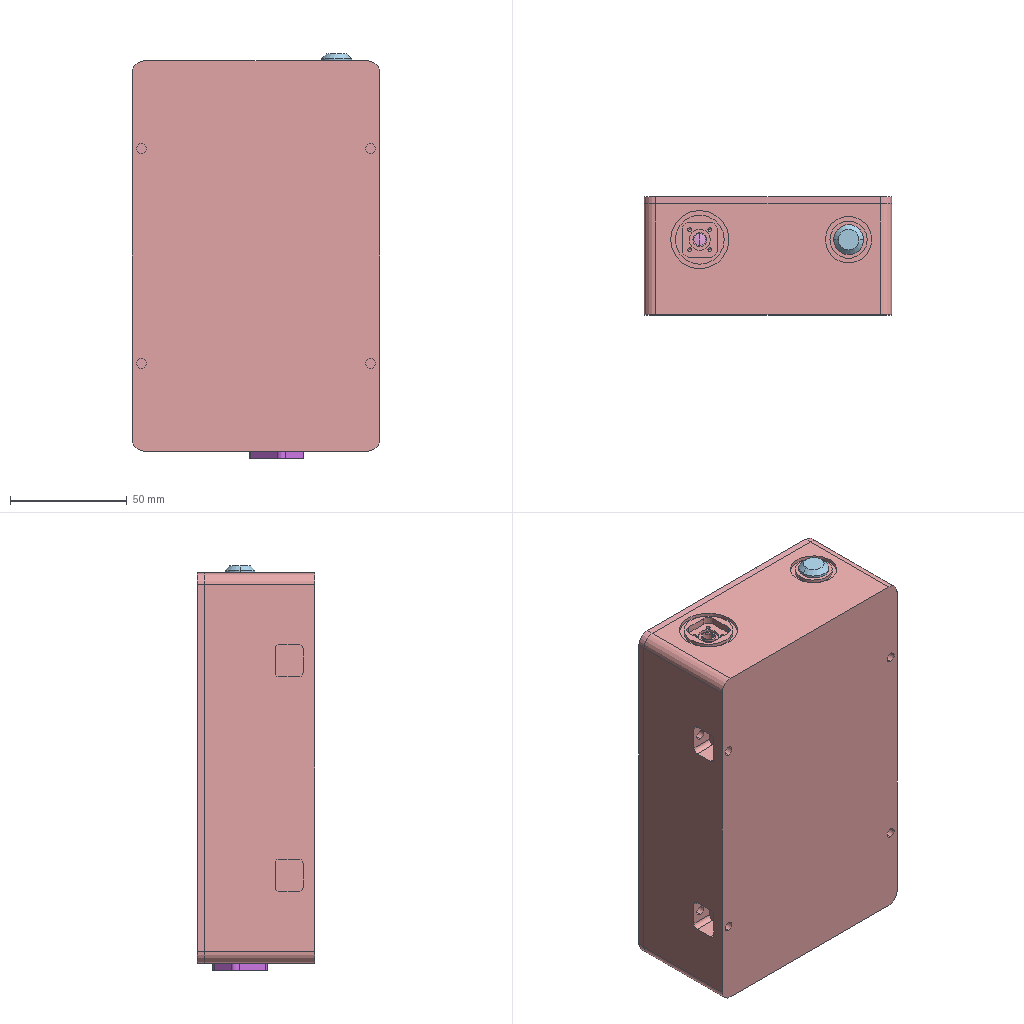Assembly | SolidWorks | 29 different items | 40 placed | box 106 x 50 x 173 mm
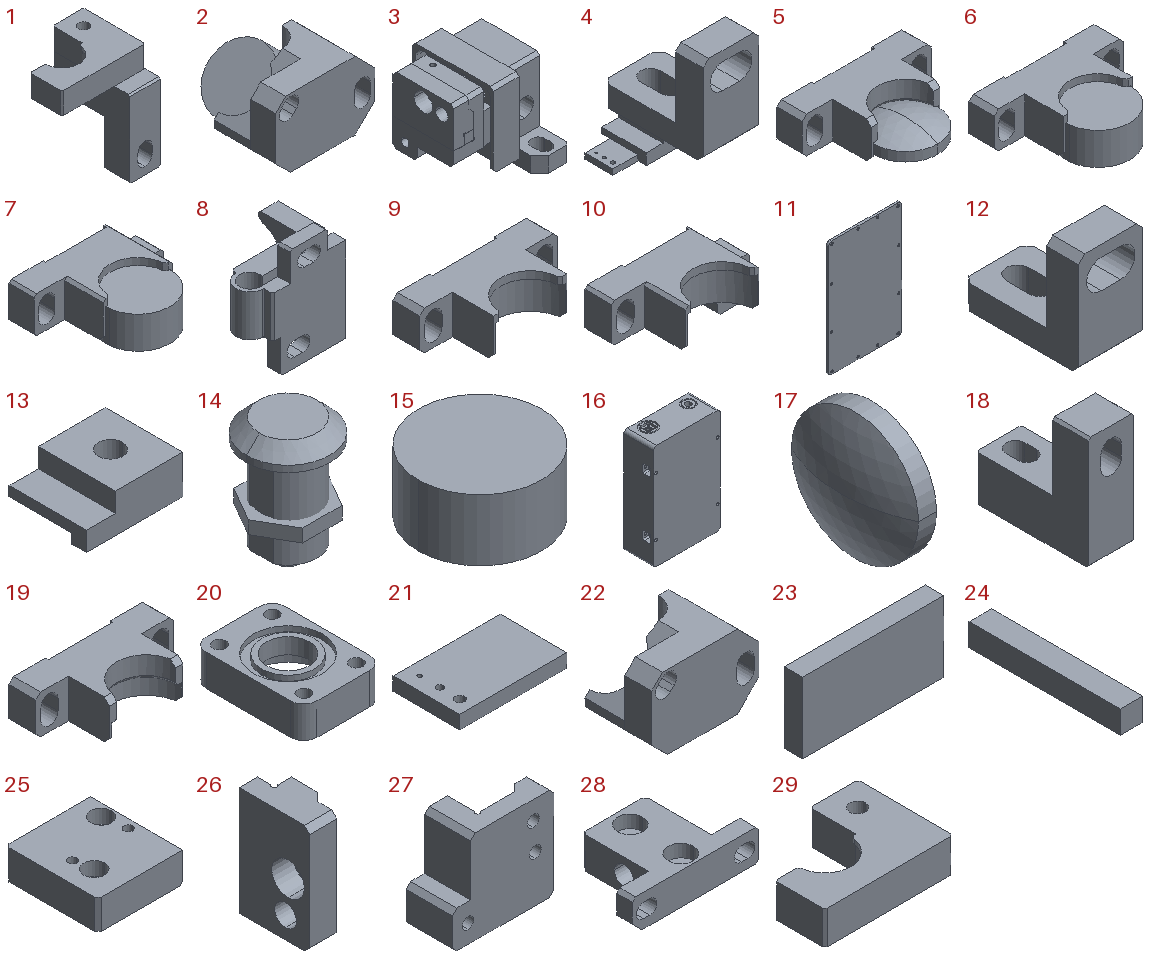Parts list (item | name | quantity | parent item | size | volume | features):
1 | (subassembly) | x1 | - | 26.9 x 25 x 32 mm | 5358 mm3 | -
2 | (subassembly) | x2 | - | 19.9 x 19.05 x 14.189 mm | 2294 mm3 | -
3 | (subassembly) | x1 | - | 27.5 x 40 x 26.65 mm | 12052 mm3 | -
4 | (subassembly) | x1 | - | 16 x 18 x 19.75 mm | 1298 mm3 | -
5 | (subassembly) | x2 | - | 25.6 x 19.05 x 7.31 mm | 1491 mm3 | features CompositeCurve 1
6 | (subassembly) | x2 | - | 25.6 x 19.05 x 7.7 mm | 1838 mm3 | -
7 | (subassembly) | x1 | - | 25.6 x 19.05 x 12.05 mm | 1859 mm3 | -
8 | - | x1 | - | 20.78 x 16.7 x 25 mm | 2347 mm3 | features MoveFace 8, Chamfer 5, ICE 5, BaseBody 1, DelFace 1, Fillet 1
9 | - | x2 | in 6 | 25.6 x 12.7 x 7.2 mm | 1033 mm3 | features ICE 7, Chamfer 3, MoveFace 2, Extrusion 1
10 | - | x1 | in 7 | 25.6 x 12.7 x 12.05 mm | 1054 mm3 | features ICE 7, Chamfer 4, MoveFace 2, Extrusion 1, Fillet 1
11 | - | x1 | - | 106 x 3 x 167 mm | 52528 mm3 | features Extrusion 1, HoleWzd 1
12 | - | x1 | in 4 | 10 x 18 x 15.75 mm | 1032 mm3 | features ICE 4, Chamfer 1, Extrusion 1
13 | - | x1 | in 4 | 10 x 8 x 4 mm | 226.365 mm3 | features ICE 4, Extrusion 1, HoleWzd 1, MoveFace 1
14 | - | x1 | - | 12.9 x 12.9 x 19.1 mm | 1271 mm3 | features ICE 4, Chamfer 1, Extrusion 1
15 | - | x5 | in 2, 6, 7 | 12.7 x 12.7 x 6.35 mm | 804.398 mm3 | features Extrusion 1
16 | - | x1 | - | 106 x 47.3 x 167 mm | 437913 mm3 | features ICE 29, MoveFace 24, HoleWzd 23, Fillet 19, Cut 18, DelFace 18, 3DProfileFeature 1, Extrusion 1, LPattern 1
17 | - | x2 | in 5 | 4.7 x 12.7 x 12.7 mm | 415.033 mm3 | features Revolution 1
18 | - | x1 | in 1 | 10 x 25 x 25 mm | 3226 mm3 | features ICE 3, Chamfer 1, Extrusion 1, MoveFace 1
19 | - | x2 | in 5 | 25.6 x 12.7 x 7.2 mm | 1076 mm3 | features ICE 7, Chamfer 2, MoveFace 2, Extrusion 1, Fillet 1
20 | - | x1 | - | 15 x 21 x 6 mm | 975.148 mm3 | features ICE 5, Extrusion 1, Fillet 1
21 | - | x1 | in 4 | 8 x 5 x 1 mm | 39.348 mm3 | features ICE 2, Extrusion 1
22 | - | x2 | in 2 | 19.9 x 12.7 x 13.659 mm | 1490 mm3 | features ICE 10, Chamfer 3, Extrusion 1, MoveFace 1
23 | - | x1 | in 3 | 20 x 2.6 x 10 mm | 520 mm3 | features Extrusion 1
24 | - | x1 | in 3 | 3 x 20 x 3 mm | 180 mm3 | features Extrusion 1
25 | - | x1 | in 3 | 24.4 x 26.5 x 8.5 mm | 3196 mm3 | features MoveFace 4, Chamfer 2, DelFace 2, HoleWzd 2, Extrusion 1, Fillet 1, ICE 1
26 | - | x1 | in 3 | 6.5 x 13 x 20 mm | 1157 mm3 | features Cut 2, Chamfer 1, Extrusion 1, HoleWzd 1
27 | - | x1 | in 3 | 21.9 x 9.9 x 20 mm | 2171 mm3 | features HoleWzd 3, ICE 2, MoveFace 2, Chamfer 1, Extrusion 1
28 | - | x1 | in 3 | 40 x 26 x 10 mm | 4828 mm3 | features ICE 3, Chamfer 2, Extrusion 1, HoleWzd 1, MoveFace 1
29 | - | x1 | in 1 | 26.9 x 20 x 7 mm | 2132 mm3 | features Chamfer 1, Extrusion 1, Fillet 1, HoleWzd 1, ICE 1
Mates (type | each side: item.copy, entity, surface, feature):
In the top assembly
Coincident | 16.1 face plane Boss-Extrude1 | 9.1 face plane Boss-Extrude3
Coincident | 16.1 face plane Boss-Extrude1 | 9.2 face plane Boss-Extrude3
PlanarAngleDim | 9.2 face plane Boss-Extrude2 | 16.1 face plane Boss-Extrude3
Coincident | 16.1 face plane Boss-Extrude1 | 10.1 face plane Boss-Extrude3
PlanarAngleDim | 10.1 face plane Boss-Extrude2 | 16.1 face plane Boss-Extrude3
Coincident | 16.1 face plane Boss-Extrude1 | 22.1 face plane Boss-Extrude1
Coincident | 16.1 face plane Boss-Extrude1 | 22.2 face plane Boss-Extrude1
PlanarAngleDim | 22.1 face plane Boss-Extrude2 | 16.1 face plane Boss-Extrude3
Coincident | 16.1 face plane Boss-Extrude1 | 12.1 face plane Boss-Extrude1
Coincident | 16.1 face plane Boss-Extrude1 | 19.1 face plane Boss-Extrude3
Parallel | 16.1 face plane Cut-Extrude9 | 19.1 face plane Boss-Extrude2
Coincident | 16.1 face plane Cut-Extrude21 | 20.1 face plane Boss-Extrude1
Concentric | 16.1 face cylinder Cut-Extrude20 | 20.1 face cylinder Boss-Extrude1
Concentric | 16.1 face cylinder Cut-Extrude27 | 14.1 face cylinder Boss-Extrude2
Coincident | 16.1 face plane Boss-Extrude3 | 14.1 face plane Boss-Extrude1
Parallel | 16.1 face plane Cut-Extrude27 | 14.1 face plane Cut-Extrude2
Parallel | 16.1 face plane Boss-Extrude1 | 26.1 face plane Boss-Extrude1
DistanceDim | 24.1 select_type:25 | 16.1 face plane Boss-Extrude1
Parallel | 16.1 face plane Cut-Extrude9 | 24.1 face plane Boss-Extrude1
Concentric | 17.1 face cylinder Revolve4 | 8.1 face cylinder Input 1
Parallel | 16.1 face plane Boss-Extrude1 | 8.1 face plane Input 1
Coincident | 17.1 face sphere Revolve4 | 8.1 vertex
Concentric | 17.2 face cylinder Revolve4 | 29.1 face cylinder Boss-Extrude1
Tangent | 17.2 face sphere Revolve4 | 29.1 face plane Boss-Extrude1
Coincident | 16.1 face plane Boss-Extrude3 | 11.1 face plane Boss-Extrude1
In subassembly 1
Coincident | 29.2 face plane Boss-Extrude1 | 18.1 face plane Boss-Extrude1 | 3 times
In subassembly 5
Concentric | 19.2 face cylinder Cut-Extrude2 | 17.3 face cylinder Revolve4
Tangent | 19.2 edge | 17.3 face sphere Revolve4
In subassembly 3
DistanceDim | 24.2 face plane Boss-Extrude1 | 26.2 face plane Boss-Extrude1 | 2 times
Coincident | 24.2 face plane Boss-Extrude1 | 26.2 face plane Boss-Extrude1
Coincident | 26.2 face plane Boss-Extrude1 | 27.1 face plane Boss-Extrude1 | 2 times
Coincident | 24.2 face plane Boss-Extrude1 | 27.1 face plane Boss-Extrude1
Coincident | 27.1 face plane Boss-Extrude1 | 23.1 face plane Boss-Extrude1 | 2 times
Coincident | 23.1 face plane Boss-Extrude1 | 25.1 face plane Boss-Extrude1
Coincident | 25.1 face plane Boss-Extrude1 | 28.1 face plane Boss-Extrude1
Width | 28.1 face plane Boss-Extrude1 | 28.1 face plane Boss-Extrude1 | 25.1 face plane Boss-Extrude1 | 25.1 face plane Boss-Extrude1
DistanceDim | 3.1 plane | 28.1 face plane Boss-Extrude1
Coincident | 27.1 face plane Boss-Extrude3 | 25.1 face plane Boss-Extrude1
DistanceDim | 27.1 face plane Boss-Extrude1 | 25.1 face plane Boss-Extrude2
In subassembly 2
Concentric | 22.3 face cylinder Cut-Extrude2 | 15.1 face cylinder Boss-Extrude1
Coincident | 22.3 face plane Cut-Extrude2 | 15.1 face plane Boss-Extrude1
In subassembly 6
Concentric | 9.3 face cylinder Cut-Extrude2 | 15.1 face cylinder Boss-Extrude1
Coincident | 9.3 face plane Cut-Extrude2 | 15.1 face plane Boss-Extrude1
In subassembly 4
Coincident | 12.2 face plane Boss-Extrude1 | 13.1 face plane Boss-Extrude2
Concentric | 13.1 face cylinder M3 Tapped Hole4 | 12.2 select_type:25
Coincident | 13.1 face plane Cut-Extrude2 | 21.1 face plane Boss-Extrude1
Coincident | 13.1 face plane Cut-Extrude2 | 21.1 face plane Cut-Extrude2
Parallel | 12.2 face plane Boss-Extrude1 | 13.1 face plane Boss-Extrude1
DistanceDim | 21.1 face plane Boss-Extrude1 | 13.1 face plane Cut-Extrude2
In subassembly 7
Concentric | 10.2 face cylinder Cut-Extrude2 | 15.1 face cylinder Boss-Extrude1
Coincident | 10.2 face plane Cut-Extrude2 | 15.1 face plane Boss-Extrude1